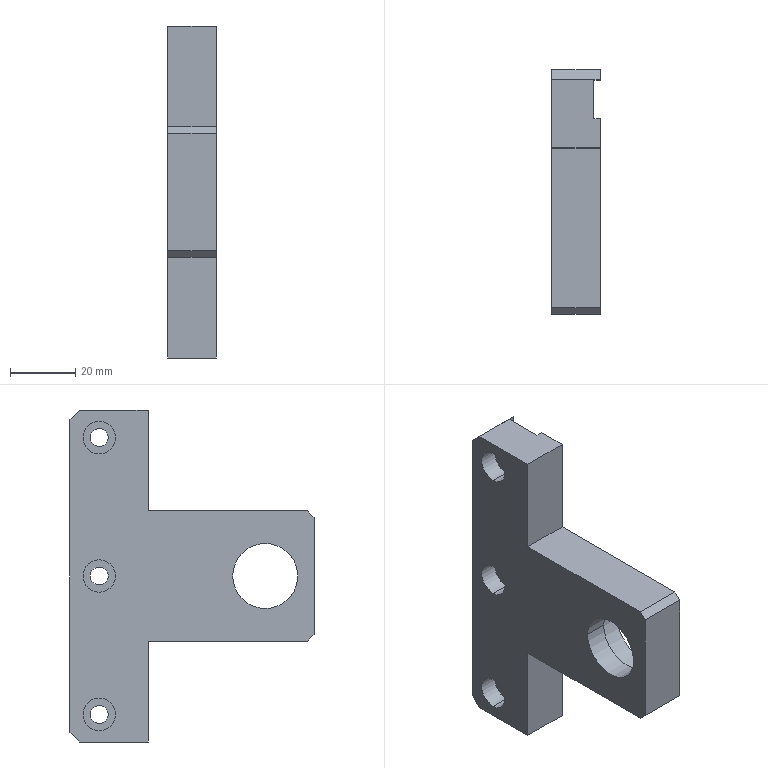Part | SolidWorks | features BaseBody 1 | 1 solid | 38 faces | box 15 x 75 x 102 mm | volume 56367 mm3 | plane 22 | cylinder 16 | commonest cylinder face diameters 5.5 x6 10 x6 20 x2 26 x2
STEP:
#1=CARTESIAN_POINT('',(-3.,-35.,-51.));
#2=VERTEX_POINT('',#1);
#3=CARTESIAN_POINT('',(-3.,-15.,-51.));
#4=VERTEX_POINT('',#3);
#5=CARTESIAN_POINT('',(-3.,-25.,-51.));
#6=DIRECTION('',(1.,0.,0.));
#7=DIRECTION('',(0.,1.,0.));
#8=AXIS2_PLACEMENT_3D('',#5,#6,#7);
#9=CIRCLE('',#8,10.);
#10=EDGE_CURVE('',#2,#4,#9,.T.);
#11=ORIENTED_EDGE('',*,*,#10,.F.);
#12=CARTESIAN_POINT('',(4.,-35.,-51.));
#13=VERTEX_POINT('',#12);
#14=CARTESIAN_POINT('',(-3.,-35.,-51.));
#15=DIRECTION('',(1.,0.,0.));
#16=VECTOR('',#15,1000.);
#17=LINE('',#14,#16);
#18=EDGE_CURVE('',#2,#13,#17,.T.);
#19=ORIENTED_EDGE('',*,*,#18,.T.);
#20=CARTESIAN_POINT('',(4.,-15.,-51.));
#21=VERTEX_POINT('',#20);
#22=CARTESIAN_POINT('',(4.,-25.,-51.));
#23=DIRECTION('',(-1.,0.,0.));
#24=DIRECTION('',(0.,1.,0.));
#25=AXIS2_PLACEMENT_3D('',#22,#23,#24);
#26=CIRCLE('',#25,10.);
#27=EDGE_CURVE('',#21,#13,#26,.T.);
#28=ORIENTED_EDGE('',*,*,#27,.F.);
#29=CARTESIAN_POINT('',(-3.,-15.,-51.));
#30=DIRECTION('',(1.,0.,0.));
#31=VECTOR('',#30,1000.);
#32=LINE('',#29,#31);
#33=EDGE_CURVE('',#4,#21,#32,.T.);
#34=ORIENTED_EDGE('',*,*,#33,.F.);
#35=EDGE_LOOP('',(#11,#19,#28,#34));
#36=FACE_OUTER_BOUND('',#35,.T.);
#37=CARTESIAN_POINT('',(-3.,-25.,-51.));
#38=DIRECTION('',(1.,0.,0.));
#39=DIRECTION('',(0.,1.,0.));
#40=AXIS2_PLACEMENT_3D('',#37,#38,#39);
#41=CYLINDRICAL_SURFACE('',#40,10.);
#42=ADVANCED_FACE('',(#36),#41,.F.);
#43=CARTESIAN_POINT('',(2.7,26.,-13.5));
#44=VERTEX_POINT('',#43);
#45=CARTESIAN_POINT('',(2.7,26.,-3.5));
#46=VERTEX_POINT('',#45);
#47=CARTESIAN_POINT('',(2.7,26.,-8.5));
#48=DIRECTION('',(-1.,0.,0.));
#49=DIRECTION('',(0.,0.,1.));
#50=AXIS2_PLACEMENT_3D('',#47,#48,#49);
#51=CIRCLE('',#50,5.);
#52=EDGE_CURVE('',#44,#46,#51,.T.);
#53=ORIENTED_EDGE('',*,*,#52,.F.);
#54=CARTESIAN_POINT('',(-3.,26.,-13.5));
#55=VERTEX_POINT('',#54);
#56=CARTESIAN_POINT('',(-3.,26.,-13.5));
#57=DIRECTION('',(-1.,0.,0.));
#58=VECTOR('',#57,1000.);
#59=LINE('',#56,#58);
#60=EDGE_CURVE('',#44,#55,#59,.T.);
#61=ORIENTED_EDGE('',*,*,#60,.T.);
#62=CARTESIAN_POINT('',(-3.,26.,-3.5));
#63=VERTEX_POINT('',#62);
#64=CARTESIAN_POINT('',(-3.,26.,-8.5));
#65=DIRECTION('',(1.,0.,0.));
#66=DIRECTION('',(0.,0.,1.));
#67=AXIS2_PLACEMENT_3D('',#64,#65,#66);
#68=CIRCLE('',#67,5.);
#69=EDGE_CURVE('',#63,#55,#68,.T.);
#70=ORIENTED_EDGE('',*,*,#69,.F.);
#71=CARTESIAN_POINT('',(-3.,26.,-3.5));
#72=DIRECTION('',(-1.,0.,0.));
#73=VECTOR('',#72,1000.);
#74=LINE('',#71,#73);
#75=EDGE_CURVE('',#46,#63,#74,.T.);
#76=ORIENTED_EDGE('',*,*,#75,.F.);
#77=EDGE_LOOP('',(#53,#61,#70,#76));
#78=FACE_OUTER_BOUND('',#77,.T.);
#79=CARTESIAN_POINT('',(-3.,26.,-8.5));
#80=DIRECTION('',(-1.,0.,0.));
#81=DIRECTION('',(0.,0.,1.));
#82=AXIS2_PLACEMENT_3D('',#79,#80,#81);
#83=CYLINDRICAL_SURFACE('',#82,5.);
#84=ADVANCED_FACE('',(#78),#83,.F.);
#85=CARTESIAN_POINT('',(2.7,26.,-56.));
#86=VERTEX_POINT('',#85);
#87=CARTESIAN_POINT('',(2.7,26.,-46.));
#88=VERTEX_POINT('',#87);
#89=CARTESIAN_POINT('',(2.7,26.,-51.));
#90=DIRECTION('',(-1.,0.,0.));
#91=DIRECTION('',(0.,0.,1.));
#92=AXIS2_PLACEMENT_3D('',#89,#90,#91);
#93=CIRCLE('',#92,5.);
#94=EDGE_CURVE('',#86,#88,#93,.T.);
#95=ORIENTED_EDGE('',*,*,#94,.F.);
#96=CARTESIAN_POINT('',(-3.,26.,-56.));
#97=VERTEX_POINT('',#96);
#98=CARTESIAN_POINT('',(-3.,26.,-56.));
#99=DIRECTION('',(-1.,0.,0.));
#100=VECTOR('',#99,1000.);
#101=LINE('',#98,#100);
#102=EDGE_CURVE('',#86,#97,#101,.T.);
#103=ORIENTED_EDGE('',*,*,#102,.T.);
#104=CARTESIAN_POINT('',(-3.,26.,-46.));
#105=VERTEX_POINT('',#104);
#106=CARTESIAN_POINT('',(-3.,26.,-51.));
#107=DIRECTION('',(1.,0.,0.));
#108=DIRECTION('',(0.,0.,1.));
#109=AXIS2_PLACEMENT_3D('',#106,#107,#108);
#110=CIRCLE('',#109,5.);
#111=EDGE_CURVE('',#105,#97,#110,.T.);
#112=ORIENTED_EDGE('',*,*,#111,.F.);
#113=CARTESIAN_POINT('',(-3.,26.,-46.));
#114=DIRECTION('',(-1.,0.,0.));
#115=VECTOR('',#114,1000.);
#116=LINE('',#113,#115);
#117=EDGE_CURVE('',#88,#105,#116,.T.);
#118=ORIENTED_EDGE('',*,*,#117,.F.);
#119=EDGE_LOOP('',(#95,#103,#112,#118));
#120=FACE_OUTER_BOUND('',#119,.T.);
#121=CARTESIAN_POINT('',(-3.,26.,-51.));
#122=DIRECTION('',(-1.,0.,0.));
#123=DIRECTION('',(0.,0.,1.));
#124=AXIS2_PLACEMENT_3D('',#121,#122,#123);
#125=CYLINDRICAL_SURFACE('',#124,5.);
#126=ADVANCED_FACE('',(#120),#125,.F.);
#127=CARTESIAN_POINT('',(2.7,26.,-98.5));
#128=VERTEX_POINT('',#127);
#129=CARTESIAN_POINT('',(2.7,26.,-88.5));
#130=VERTEX_POINT('',#129);
#131=CARTESIAN_POINT('',(2.7,26.,-93.5));
#132=DIRECTION('',(-1.,0.,0.));
#133=DIRECTION('',(0.,0.,1.));
#134=AXIS2_PLACEMENT_3D('',#131,#132,#133);
#135=CIRCLE('',#134,5.);
#136=EDGE_CURVE('',#128,#130,#135,.T.);
#137=ORIENTED_EDGE('',*,*,#136,.F.);
#138=CARTESIAN_POINT('',(-3.,26.,-98.5));
#139=VERTEX_POINT('',#138);
#140=CARTESIAN_POINT('',(-3.,26.,-98.5));
#141=DIRECTION('',(-1.,0.,0.));
#142=VECTOR('',#141,1000.);
#143=LINE('',#140,#142);
#144=EDGE_CURVE('',#128,#139,#143,.T.);
#145=ORIENTED_EDGE('',*,*,#144,.T.);
#146=CARTESIAN_POINT('',(-3.,26.,-88.5));
#147=VERTEX_POINT('',#146);
#148=CARTESIAN_POINT('',(-3.,26.,-93.5));
#149=DIRECTION('',(1.,0.,0.));
#150=DIRECTION('',(0.,0.,1.));
#151=AXIS2_PLACEMENT_3D('',#148,#149,#150);
#152=CIRCLE('',#151,5.);
#153=EDGE_CURVE('',#147,#139,#152,.T.);
#154=ORIENTED_EDGE('',*,*,#153,.F.);
#155=CARTESIAN_POINT('',(-3.,26.,-88.5));
#156=DIRECTION('',(-1.,0.,0.));
#157=VECTOR('',#156,1000.);
#158=LINE('',#155,#157);
#159=EDGE_CURVE('',#130,#147,#158,.T.);
#160=ORIENTED_EDGE('',*,*,#159,.F.);
#161=EDGE_LOOP('',(#137,#145,#154,#160));
#162=FACE_OUTER_BOUND('',#161,.T.);
#163=CARTESIAN_POINT('',(-3.,26.,-93.5));
#164=DIRECTION('',(-1.,0.,0.));
#165=DIRECTION('',(0.,0.,1.));
#166=AXIS2_PLACEMENT_3D('',#163,#164,#165);
#167=CYLINDRICAL_SURFACE('',#166,5.);
#168=ADVANCED_FACE('',(#162),#167,.F.);
#169=CARTESIAN_POINT('',(4.,-38.,-51.));
#170=VERTEX_POINT('',#169);
#171=CARTESIAN_POINT('',(4.,-12.,-51.));
#172=VERTEX_POINT('',#171);
#173=CARTESIAN_POINT('',(4.,-25.,-51.));
#174=DIRECTION('',(1.,0.,0.));
#175=DIRECTION('',(0.,1.,0.));
#176=AXIS2_PLACEMENT_3D('',#173,#174,#175);
#177=CIRCLE('',#176,13.);
#178=EDGE_CURVE('',#170,#172,#177,.T.);
#179=ORIENTED_EDGE('',*,*,#178,.F.);
#180=CARTESIAN_POINT('',(12.,-38.,-51.));
#181=VERTEX_POINT('',#180);
#182=CARTESIAN_POINT('',(4.,-38.,-51.));
#183=DIRECTION('',(1.,0.,0.));
#184=VECTOR('',#183,1000.);
#185=LINE('',#182,#184);
#186=EDGE_CURVE('',#170,#181,#185,.T.);
#187=ORIENTED_EDGE('',*,*,#186,.T.);
#188=CARTESIAN_POINT('',(12.,-12.,-51.));
#189=VERTEX_POINT('',#188);
#190=CARTESIAN_POINT('',(12.,-25.,-51.));
#191=DIRECTION('',(-1.,0.,0.));
#192=DIRECTION('',(0.,1.,0.));
#193=AXIS2_PLACEMENT_3D('',#190,#191,#192);
#194=CIRCLE('',#193,13.);
#195=EDGE_CURVE('',#189,#181,#194,.T.);
#196=ORIENTED_EDGE('',*,*,#195,.F.);
#197=CARTESIAN_POINT('',(4.,-12.,-51.));
#198=DIRECTION('',(1.,0.,0.));
#199=VECTOR('',#198,1000.);
#200=LINE('',#197,#199);
#201=EDGE_CURVE('',#172,#189,#200,.T.);
#202=ORIENTED_EDGE('',*,*,#201,.F.);
#203=EDGE_LOOP('',(#179,#187,#196,#202));
#204=FACE_OUTER_BOUND('',#203,.T.);
#205=CARTESIAN_POINT('',(4.,-25.,-51.));
#206=DIRECTION('',(1.,0.,0.));
#207=DIRECTION('',(0.,1.,0.));
#208=AXIS2_PLACEMENT_3D('',#205,#206,#207);
#209=CYLINDRICAL_SURFACE('',#208,13.);
#210=ADVANCED_FACE('',(#204),#209,.F.);
#211=CARTESIAN_POINT('',(10.,26.,-5.75));
#212=VERTEX_POINT('',#211);
#213=CARTESIAN_POINT('',(10.,26.,-11.25));
#214=VERTEX_POINT('',#213);
#215=CARTESIAN_POINT('',(10.,26.,-8.5));
#216=DIRECTION('',(1.,0.,0.));
#217=DIRECTION('',(0.,0.,1.));
#218=AXIS2_PLACEMENT_3D('',#215,#216,#217);
#219=CIRCLE('',#218,2.75);
#220=EDGE_CURVE('',#212,#214,#219,.T.);
#221=ORIENTED_EDGE('',*,*,#220,.T.);
#222=CARTESIAN_POINT('',(2.7,26.,-11.25));
#223=VERTEX_POINT('',#222);
#224=CARTESIAN_POINT('',(-3.,26.,-11.25));
#225=DIRECTION('',(-1.,0.,0.));
#226=VECTOR('',#225,1000.);
#227=LINE('',#224,#226);
#228=EDGE_CURVE('',#214,#223,#227,.T.);
#229=ORIENTED_EDGE('',*,*,#228,.T.);
#230=CARTESIAN_POINT('',(2.7,26.,-5.75));
#231=VERTEX_POINT('',#230);
#232=CARTESIAN_POINT('',(2.7,26.,-8.5));
#233=DIRECTION('',(-1.,0.,0.));
#234=DIRECTION('',(0.,0.,1.));
#235=AXIS2_PLACEMENT_3D('',#232,#233,#234);
#236=CIRCLE('',#235,2.75);
#237=EDGE_CURVE('',#223,#231,#236,.T.);
#238=ORIENTED_EDGE('',*,*,#237,.T.);
#239=CARTESIAN_POINT('',(-3.,26.,-5.75));
#240=DIRECTION('',(-1.,0.,0.));
#241=VECTOR('',#240,1000.);
#242=LINE('',#239,#241);
#243=EDGE_CURVE('',#212,#231,#242,.T.);
#244=ORIENTED_EDGE('',*,*,#243,.F.);
#245=EDGE_LOOP('',(#221,#229,#238,#244));
#246=FACE_OUTER_BOUND('',#245,.T.);
#247=CARTESIAN_POINT('',(-3.,26.,-8.5));
#248=DIRECTION('',(-1.,0.,0.));
#249=DIRECTION('',(0.,0.,1.));
#250=AXIS2_PLACEMENT_3D('',#247,#248,#249);
#251=CYLINDRICAL_SURFACE('',#250,2.75);
#252=ADVANCED_FACE('',(#246),#251,.F.);
#253=CARTESIAN_POINT('',(10.,26.,-48.25));
#254=VERTEX_POINT('',#253);
#255=CARTESIAN_POINT('',(10.,26.,-53.75));
#256=VERTEX_POINT('',#255);
#257=CARTESIAN_POINT('',(10.,26.,-51.));
#258=DIRECTION('',(1.,0.,0.));
#259=DIRECTION('',(0.,0.,1.));
#260=AXIS2_PLACEMENT_3D('',#257,#258,#259);
#261=CIRCLE('',#260,2.75);
#262=EDGE_CURVE('',#254,#256,#261,.T.);
#263=ORIENTED_EDGE('',*,*,#262,.T.);
#264=CARTESIAN_POINT('',(2.7,26.,-53.75));
#265=VERTEX_POINT('',#264);
#266=CARTESIAN_POINT('',(-3.,26.,-53.75));
#267=DIRECTION('',(-1.,0.,0.));
#268=VECTOR('',#267,1000.);
#269=LINE('',#266,#268);
#270=EDGE_CURVE('',#256,#265,#269,.T.);
#271=ORIENTED_EDGE('',*,*,#270,.T.);
#272=CARTESIAN_POINT('',(2.7,26.,-48.25));
#273=VERTEX_POINT('',#272);
#274=CARTESIAN_POINT('',(2.7,26.,-51.));
#275=DIRECTION('',(-1.,0.,0.));
#276=DIRECTION('',(0.,0.,1.));
#277=AXIS2_PLACEMENT_3D('',#274,#275,#276);
#278=CIRCLE('',#277,2.75);
#279=EDGE_CURVE('',#265,#273,#278,.T.);
#280=ORIENTED_EDGE('',*,*,#279,.T.);
#281=CARTESIAN_POINT('',(-3.,26.,-48.25));
#282=DIRECTION('',(-1.,0.,0.));
#283=VECTOR('',#282,1000.);
#284=LINE('',#281,#283);
#285=EDGE_CURVE('',#254,#273,#284,.T.);
#286=ORIENTED_EDGE('',*,*,#285,.F.);
#287=EDGE_LOOP('',(#263,#271,#280,#286));
#288=FACE_OUTER_BOUND('',#287,.T.);
#289=CARTESIAN_POINT('',(-3.,26.,-51.));
#290=DIRECTION('',(-1.,0.,0.));
#291=DIRECTION('',(0.,0.,1.));
#292=AXIS2_PLACEMENT_3D('',#289,#290,#291);
#293=CYLINDRICAL_SURFACE('',#292,2.75);
#294=ADVANCED_FACE('',(#288),#293,.F.);
#295=CARTESIAN_POINT('',(10.,26.,-90.75));
#296=VERTEX_POINT('',#295);
#297=CARTESIAN_POINT('',(10.,26.,-96.25));
#298=VERTEX_POINT('',#297);
#299=CARTESIAN_POINT('',(10.,26.,-93.5));
#300=DIRECTION('',(1.,0.,0.));
#301=DIRECTION('',(0.,0.,1.));
#302=AXIS2_PLACEMENT_3D('',#299,#300,#301);
#303=CIRCLE('',#302,2.75);
#304=EDGE_CURVE('',#296,#298,#303,.T.);
#305=ORIENTED_EDGE('',*,*,#304,.T.);
#306=CARTESIAN_POINT('',(2.7,26.,-96.25));
#307=VERTEX_POINT('',#306);
#308=CARTESIAN_POINT('',(-3.,26.,-96.25));
#309=DIRECTION('',(-1.,0.,0.));
#310=VECTOR('',#309,1000.);
#311=LINE('',#308,#310);
#312=EDGE_CURVE('',#298,#307,#311,.T.);
#313=ORIENTED_EDGE('',*,*,#312,.T.);
#314=CARTESIAN_POINT('',(2.7,26.,-90.75));
#315=VERTEX_POINT('',#314);
#316=CARTESIAN_POINT('',(2.7,26.,-93.5));
#317=DIRECTION('',(-1.,0.,0.));
#318=DIRECTION('',(0.,0.,1.));
#319=AXIS2_PLACEMENT_3D('',#316,#317,#318);
#320=CIRCLE('',#319,2.75);
#321=EDGE_CURVE('',#307,#315,#320,.T.);
#322=ORIENTED_EDGE('',*,*,#321,.T.);
#323=CARTESIAN_POINT('',(-3.,26.,-90.75));
#324=DIRECTION('',(-1.,0.,0.));
#325=VECTOR('',#324,1000.);
#326=LINE('',#323,#325);
#327=EDGE_CURVE('',#296,#315,#326,.T.);
#328=ORIENTED_EDGE('',*,*,#327,.F.);
#329=EDGE_LOOP('',(#305,#313,#322,#328));
#330=FACE_OUTER_BOUND('',#329,.T.);
#331=CARTESIAN_POINT('',(-3.,26.,-93.5));
#332=DIRECTION('',(-1.,0.,0.));
#333=DIRECTION('',(0.,0.,1.));
#334=AXIS2_PLACEMENT_3D('',#331,#332,#333);
#335=CYLINDRICAL_SURFACE('',#334,2.75);
#336=ADVANCED_FACE('',(#330),#335,.F.);
#337=CARTESIAN_POINT('',(-3.,-25.,-51.));
#338=DIRECTION('',(1.,0.,0.));
#339=DIRECTION('',(0.,1.,0.));
#340=AXIS2_PLACEMENT_3D('',#337,#338,#339);
#341=CIRCLE('',#340,10.);
#342=EDGE_CURVE('',#4,#2,#341,.T.);
#343=ORIENTED_EDGE('',*,*,#342,.T.);
#344=ORIENTED_EDGE('',*,*,#10,.T.);
#345=EDGE_LOOP('',(#343,#344));
#346=FACE_BOUND('',#345,.T.);
#347=ORIENTED_EDGE('',*,*,#69,.T.);
#348=CARTESIAN_POINT('',(-3.,26.,-8.5));
#349=DIRECTION('',(1.,0.,0.));
#350=DIRECTION('',(0.,0.,1.));
#351=AXIS2_PLACEMENT_3D('',#348,#349,#350);
#352=CIRCLE('',#351,5.);
#353=EDGE_CURVE('',#55,#63,#352,.T.);
#354=ORIENTED_EDGE('',*,*,#353,.T.);
#355=EDGE_LOOP('',(#347,#354));
#356=FACE_BOUND('',#355,.T.);
#357=ORIENTED_EDGE('',*,*,#111,.T.);
#358=CARTESIAN_POINT('',(-3.,26.,-51.));
#359=DIRECTION('',(1.,0.,0.));
#360=DIRECTION('',(0.,0.,1.));
#361=AXIS2_PLACEMENT_3D('',#358,#359,#360);
#362=CIRCLE('',#361,5.);
#363=EDGE_CURVE('',#97,#105,#362,.T.);
#364=ORIENTED_EDGE('',*,*,#363,.T.);
#365=EDGE_LOOP('',(#357,#364));
#366=FACE_BOUND('',#365,.T.);
#367=ORIENTED_EDGE('',*,*,#153,.T.);
#368=CARTESIAN_POINT('',(-3.,26.,-93.5));
#369=DIRECTION('',(1.,0.,0.));
#370=DIRECTION('',(0.,0.,1.));
#371=AXIS2_PLACEMENT_3D('',#368,#369,#370);
#372=CIRCLE('',#371,5.);
#373=EDGE_CURVE('',#139,#147,#372,.T.);
#374=ORIENTED_EDGE('',*,*,#373,.T.);
#375=EDGE_LOOP('',(#367,#374));
#376=FACE_BOUND('',#375,.T.);
#377=CARTESIAN_POINT('',(-3.,11.,-71.));
#378=VERTEX_POINT('',#377);
#379=CARTESIAN_POINT('',(-3.,-38.,-71.));
#380=VERTEX_POINT('',#379);
#381=CARTESIAN_POINT('',(-3.,35.,-71.));
#382=DIRECTION('',(0.,-1.,0.));
#383=VECTOR('',#382,1000.);
#384=LINE('',#381,#383);
#385=EDGE_CURVE('',#378,#380,#384,.T.);
#386=ORIENTED_EDGE('',*,*,#385,.T.);
#387=CARTESIAN_POINT('',(-3.,-40.,-69.));
#388=VERTEX_POINT('',#387);
#389=CARTESIAN_POINT('',(-3.,-38.,-71.));
#390=DIRECTION('',(0.,-0.7071,0.7071));
#391=VECTOR('',#390,1000.);
#392=LINE('',#389,#391);
#393=EDGE_CURVE('',#380,#388,#392,.T.);
#394=ORIENTED_EDGE('',*,*,#393,.T.);
#395=CARTESIAN_POINT('',(-3.,-40.,-33.));
#396=VERTEX_POINT('',#395);
#397=CARTESIAN_POINT('',(-3.,-40.,-102.));
#398=DIRECTION('',(0.,0.,1.));
#399=VECTOR('',#398,1000.);
#400=LINE('',#397,#399);
#401=EDGE_CURVE('',#388,#396,#400,.T.);
#402=ORIENTED_EDGE('',*,*,#401,.T.);
#403=CARTESIAN_POINT('',(-3.,-38.,-31.));
#404=VERTEX_POINT('',#403);
#405=CARTESIAN_POINT('',(-3.,-40.,-33.));
#406=DIRECTION('',(0.,0.7071,0.7071));
#407=VECTOR('',#406,1000.);
#408=LINE('',#405,#407);
#409=EDGE_CURVE('',#396,#404,#408,.T.);
#410=ORIENTED_EDGE('',*,*,#409,.T.);
#411=CARTESIAN_POINT('',(-3.,11.,-31.));
#412=VERTEX_POINT('',#411);
#413=CARTESIAN_POINT('',(-3.,35.,-31.));
#414=DIRECTION('',(0.,1.,0.));
#415=VECTOR('',#414,1000.);
#416=LINE('',#413,#415);
#417=EDGE_CURVE('',#404,#412,#416,.T.);
#418=ORIENTED_EDGE('',*,*,#417,.T.);
#419=CARTESIAN_POINT('',(-3.,11.,0.));
#420=VERTEX_POINT('',#419);
#421=CARTESIAN_POINT('',(-3.,11.,-102.));
#422=DIRECTION('',(0.,0.,1.));
#423=VECTOR('',#422,1000.);
#424=LINE('',#421,#423);
#425=EDGE_CURVE('',#412,#420,#424,.T.);
#426=ORIENTED_EDGE('',*,*,#425,.T.);
#427=CARTESIAN_POINT('',(-3.,32.,0.));
#428=VERTEX_POINT('',#427);
#429=CARTESIAN_POINT('',(-3.,35.,0.));
#430=DIRECTION('',(0.,1.,0.));
#431=VECTOR('',#430,1000.);
#432=LINE('',#429,#431);
#433=EDGE_CURVE('',#420,#428,#432,.T.);
#434=ORIENTED_EDGE('',*,*,#433,.T.);
#435=CARTESIAN_POINT('',(-3.,35.,-3.));
#436=VERTEX_POINT('',#435);
#437=CARTESIAN_POINT('',(-3.,32.,0.));
#438=DIRECTION('',(0.,0.7071,-0.7071));
#439=VECTOR('',#438,1000.);
#440=LINE('',#437,#439);
#441=EDGE_CURVE('',#428,#436,#440,.T.);
#442=ORIENTED_EDGE('',*,*,#441,.T.);
#443=CARTESIAN_POINT('',(-3.,35.,-99.));
#444=VERTEX_POINT('',#443);
#445=CARTESIAN_POINT('',(-3.,35.,-102.));
#446=DIRECTION('',(0.,0.,-1.));
#447=VECTOR('',#446,1000.);
#448=LINE('',#445,#447);
#449=EDGE_CURVE('',#436,#444,#448,.T.);
#450=ORIENTED_EDGE('',*,*,#449,.T.);
#451=CARTESIAN_POINT('',(-3.,32.,-102.));
#452=VERTEX_POINT('',#451);
#453=CARTESIAN_POINT('',(-3.,35.,-99.));
#454=DIRECTION('',(0.,-0.7071,-0.7071));
#455=VECTOR('',#454,1000.);
#456=LINE('',#453,#455);
#457=EDGE_CURVE('',#444,#452,#456,.T.);
#458=ORIENTED_EDGE('',*,*,#457,.T.);
#459=CARTESIAN_POINT('',(-3.,11.,-102.));
#460=VERTEX_POINT('',#459);
#461=CARTESIAN_POINT('',(-3.,35.,-102.));
#462=DIRECTION('',(0.,-1.,0.));
#463=VECTOR('',#462,1000.);
#464=LINE('',#461,#463);
#465=EDGE_CURVE('',#452,#460,#464,.T.);
#466=ORIENTED_EDGE('',*,*,#465,.T.);
#467=CARTESIAN_POINT('',(-3.,11.,-102.));
#468=DIRECTION('',(0.,0.,1.));
#469=VECTOR('',#468,1000.);
#470=LINE('',#467,#469);
#471=EDGE_CURVE('',#460,#378,#470,.T.);
#472=ORIENTED_EDGE('',*,*,#471,.T.);
#473=EDGE_LOOP('',(#386,#394,#402,#410,#418,#426,#434,#442,#450,#458,#466,#472));
#474=FACE_OUTER_BOUND('',#473,.T.);
#475=CARTESIAN_POINT('',(-3.,35.,-102.));
#476=DIRECTION('',(-1.,0.,0.));
#477=DIRECTION('',(0.,-1.,0.));
#478=AXIS2_PLACEMENT_3D('',#475,#476,#477);
#479=PLANE('',#478);
#480=ADVANCED_FACE('',(#346,#356,#366,#376,#474),#479,.T.);
#481=ORIENTED_EDGE('',*,*,#18,.F.);
#482=ORIENTED_EDGE('',*,*,#342,.F.);
#483=ORIENTED_EDGE('',*,*,#33,.T.);
#484=CARTESIAN_POINT('',(4.,-25.,-51.));
#485=DIRECTION('',(-1.,0.,0.));
#486=DIRECTION('',(0.,1.,0.));
#487=AXIS2_PLACEMENT_3D('',#484,#485,#486);
#488=CIRCLE('',#487,10.);
#489=EDGE_CURVE('',#13,#21,#488,.T.);
#490=ORIENTED_EDGE('',*,*,#489,.F.);
#491=EDGE_LOOP('',(#481,#482,#483,#490));
#492=FACE_OUTER_BOUND('',#491,.T.);
#493=CARTESIAN_POINT('',(-3.,-25.,-51.));
#494=DIRECTION('',(1.,0.,0.));
#495=DIRECTION('',(0.,1.,0.));
#496=AXIS2_PLACEMENT_3D('',#493,#494,#495);
#497=CYLINDRICAL_SURFACE('',#496,10.);
#498=ADVANCED_FACE('',(#492),#497,.F.);
#499=ORIENTED_EDGE('',*,*,#60,.F.);
#500=CARTESIAN_POINT('',(2.7,26.,-8.5));
#501=DIRECTION('',(-1.,0.,0.));
#502=DIRECTION('',(0.,0.,1.));
#503=AXIS2_PLACEMENT_3D('',#500,#501,#502);
#504=CIRCLE('',#503,5.);
#505=EDGE_CURVE('',#46,#44,#504,.T.);
#506=ORIENTED_EDGE('',*,*,#505,.F.);
#507=ORIENTED_EDGE('',*,*,#75,.T.);
#508=ORIENTED_EDGE('',*,*,#353,.F.);
#509=EDGE_LOOP('',(#499,#506,#507,#508));
#510=FACE_OUTER_BOUND('',#509,.T.);
#511=CARTESIAN_POINT('',(-3.,26.,-8.5));
#512=DIRECTION('',(-1.,0.,0.));
#513=DIRECTION('',(0.,0.,1.));
#514=AXIS2_PLACEMENT_3D('',#511,#512,#513);
#515=CYLINDRICAL_SURFACE('',#514,5.);
#516=ADVANCED_FACE('',(#510),#515,.F.);
#517=ORIENTED_EDGE('',*,*,#102,.F.);
#518=CARTESIAN_POINT('',(2.7,26.,-51.));
#519=DIRECTION('',(-1.,0.,0.));
#520=DIRECTION('',(0.,0.,1.));
#521=AXIS2_PLACEMENT_3D('',#518,#519,#520);
#522=CIRCLE('',#521,5.);
#523=EDGE_CURVE('',#88,#86,#522,.T.);
#524=ORIENTED_EDGE('',*,*,#523,.F.);
#525=ORIENTED_EDGE('',*,*,#117,.T.);
#526=ORIENTED_EDGE('',*,*,#363,.F.);
#527=EDGE_LOOP('',(#517,#524,#525,#526));
#528=FACE_OUTER_BOUND('',#527,.T.);
#529=CARTESIAN_POINT('',(-3.,26.,-51.));
#530=DIRECTION('',(-1.,0.,0.));
#531=DIRECTION('',(0.,0.,1.));
#532=AXIS2_PLACEMENT_3D('',#529,#530,#531);
#533=CYLINDRICAL_SURFACE('',#532,5.);
#534=ADVANCED_FACE('',(#528),#533,.F.);
#535=ORIENTED_EDGE('',*,*,#144,.F.);
#536=CARTESIAN_POINT('',(2.7,26.,-93.5));
#537=DIRECTION('',(-1.,0.,0.));
#538=DIRECTION('',(0.,0.,1.));
#539=AXIS2_PLACEMENT_3D('',#536,#537,#538);
#540=CIRCLE('',#539,5.);
#541=EDGE_CURVE('',#130,#128,#540,.T.);
#542=ORIENTED_EDGE('',*,*,#541,.F.);
#543=ORIENTED_EDGE('',*,*,#159,.T.);
#544=ORIENTED_EDGE('',*,*,#373,.F.);
#545=EDGE_LOOP('',(#535,#542,#543,#544));
#546=FACE_OUTER_BOUND('',#545,.T.);
#547=CARTESIAN_POINT('',(-3.,26.,-93.5));
#548=DIRECTION('',(-1.,0.,0.));
#549=DIRECTION('',(0.,0.,1.));
#550=AXIS2_PLACEMENT_3D('',#547,#548,#549);
#551=CYLINDRICAL_SURFACE('',#550,5.);
#552=ADVANCED_FACE('',(#546),#551,.F.);
#553=ORIENTED_EDGE('',*,*,#393,.F.);
#554=CARTESIAN_POINT('',(12.,-38.,-71.));
#555=VERTEX_POINT('',#554);
#556=CARTESIAN_POINT('',(-3.,-38.,-71.));
#557=DIRECTION('',(1.,0.,0.));
#558=VECTOR('',#557,1000.);
#559=LINE('',#556,#558);
#560=EDGE_CURVE('',#380,#555,#559,.T.);
#561=ORIENTED_EDGE('',*,*,#560,.T.);
#562=CARTESIAN_POINT('',(12.,-40.,-69.));
#563=VERTEX_POINT('',#562);
#564=CARTESIAN_POINT('',(12.,-38.,-71.));
#565=DIRECTION('',(0.,-0.7071,0.7071));
#566=VECTOR('',#565,1000.);
#567=LINE('',#564,#566);
#568=EDGE_CURVE('',#555,#563,#567,.T.);
#569=ORIENTED_EDGE('',*,*,#568,.T.);
#570=CARTESIAN_POINT('',(-3.,-40.,-69.));
#571=DIRECTION('',(-1.,0.,0.));
#572=VECTOR('',#571,1000.);
#573=LINE('',#570,#572);
#574=EDGE_CURVE('',#563,#388,#573,.T.);
#575=ORIENTED_EDGE('',*,*,#574,.T.);
#576=EDGE_LOOP('',(#553,#561,#569,#575));
#577=FACE_OUTER_BOUND('',#576,.T.);
#578=CARTESIAN_POINT('',(-3.,-38.,-71.));
#579=DIRECTION('',(0.,-0.7071,-0.7071));
#580=DIRECTION('',(0.,0.7071,-0.7071));
#581=AXIS2_PLACEMENT_3D('',#578,#579,#580);
#582=PLANE('',#581);
#583=ADVANCED_FACE('',(#577),#582,.T.);
#584=ORIENTED_EDGE('',*,*,#560,.F.);
#585=ORIENTED_EDGE('',*,*,#385,.F.);
#586=CARTESIAN_POINT('',(12.,11.,-71.));
#587=VERTEX_POINT('',#586);
#588=CARTESIAN_POINT('',(-3.,11.,-71.));
#589=DIRECTION('',(-1.,0.,0.));
#590=VECTOR('',#589,1000.);
#591=LINE('',#588,#590);
#592=EDGE_CURVE('',#587,#378,#591,.T.);
#593=ORIENTED_EDGE('',*,*,#592,.F.);
#594=CARTESIAN_POINT('',(12.,11.,-71.));
#595=DIRECTION('',(0.,1.,0.));
#596=VECTOR('',#595,1000.);
#597=LINE('',#594,#596);
#598=EDGE_CURVE('',#555,#587,#597,.T.);
#599=ORIENTED_EDGE('',*,*,#598,.F.);
#600=EDGE_LOOP('',(#584,#585,#593,#599));
#601=FACE_OUTER_BOUND('',#600,.T.);
#602=CARTESIAN_POINT('',(-3.,11.,-71.));
#603=DIRECTION('',(0.,0.,1.));
#604=DIRECTION('',(0.,-1.,0.));
#605=AXIS2_PLACEMENT_3D('',#602,#603,#604);
#606=PLANE('',#605);
#607=ADVANCED_FACE('',(#601),#606,.F.);
#608=ORIENTED_EDGE('',*,*,#592,.T.);
#609=ORIENTED_EDGE('',*,*,#471,.F.);
#610=CARTESIAN_POINT('',(12.,11.,-102.));
#611=VERTEX_POINT('',#610);
#612=CARTESIAN_POINT('',(-3.,11.,-102.));
#613=DIRECTION('',(-1.,0.,0.));
#614=VECTOR('',#613,1000.);
#615=LINE('',#612,#614);
#616=EDGE_CURVE('',#611,#460,#615,.T.);
#617=ORIENTED_EDGE('',*,*,#616,.F.);
#618=CARTESIAN_POINT('',(12.,11.,-102.));
#619=DIRECTION('',(0.,0.,-1.));
#620=VECTOR('',#619,1000.);
#621=LINE('',#618,#620);
#622=EDGE_CURVE('',#587,#611,#621,.T.);
#623=ORIENTED_EDGE('',*,*,#622,.F.);
#624=EDGE_LOOP('',(#608,#609,#617,#623));
#625=FACE_OUTER_BOUND('',#624,.T.);
#626=CARTESIAN_POINT('',(-3.,11.,-102.));
#627=DIRECTION('',(0.,1.,0.));
#628=DIRECTION('',(-1.,0.,0.));
#629=AXIS2_PLACEMENT_3D('',#626,#627,#628);
#630=PLANE('',#629);
#631=ADVANCED_FACE('',(#625),#630,.F.);
#632=ORIENTED_EDGE('',*,*,#616,.T.);
#633=ORIENTED_EDGE('',*,*,#465,.F.);
#634=CARTESIAN_POINT('',(10.,32.,-102.));
#635=VERTEX_POINT('',#634);
#636=CARTESIAN_POINT('',(0.,32.,-102.));
#637=DIRECTION('',(-1.,0.,0.));
#638=VECTOR('',#637,1000.);
#639=LINE('',#636,#638);
#640=EDGE_CURVE('',#635,#452,#639,.T.);
#641=ORIENTED_EDGE('',*,*,#640,.F.);
#642=CARTESIAN_POINT('',(10.,20.,-102.));
#643=VERTEX_POINT('',#642);
#644=CARTESIAN_POINT('',(10.,0.,-102.));
#645=DIRECTION('',(0.,1.,0.));
#646=VECTOR('',#645,1000.);
#647=LINE('',#644,#646);
#648=EDGE_CURVE('',#643,#635,#647,.T.);
#649=ORIENTED_EDGE('',*,*,#648,.F.);
#650=CARTESIAN_POINT('',(12.,20.,-102.));
#651=VERTEX_POINT('',#650);
#652=CARTESIAN_POINT('',(0.,20.,-102.));
#653=DIRECTION('',(-1.,0.,0.));
#654=VECTOR('',#653,1000.);
#655=LINE('',#652,#654);
#656=EDGE_CURVE('',#651,#643,#655,.T.);
#657=ORIENTED_EDGE('',*,*,#656,.F.);
#658=CARTESIAN_POINT('',(12.,0.,-102.));
#659=DIRECTION('',(0.,1.,0.));
#660=VECTOR('',#659,1000.);
#661=LINE('',#658,#660);
#662=EDGE_CURVE('',#611,#651,#661,.T.);
#663=ORIENTED_EDGE('',*,*,#662,.F.);
#664=EDGE_LOOP('',(#632,#633,#641,#649,#657,#663));
#665=FACE_OUTER_BOUND('',#664,.T.);
#666=CARTESIAN_POINT('',(0.,0.,-102.));
#667=DIRECTION('',(0.,0.,1.));
#668=DIRECTION('',(1.,0.,0.));
#669=AXIS2_PLACEMENT_3D('',#666,#667,#668);
#670=PLANE('',#669);
#671=ADVANCED_FACE('',(#665),#670,.F.);
#672=CARTESIAN_POINT('',(12.,35.,-99.));
#673=VERTEX_POINT('',#672);
#674=CARTESIAN_POINT('',(-3.,35.,-99.));
#675=DIRECTION('',(1.,0.,0.));
#676=VECTOR('',#675,1000.);
#677=LINE('',#674,#676);
#678=EDGE_CURVE('',#444,#673,#677,.T.);
#679=ORIENTED_EDGE('',*,*,#678,.T.);
#680=CARTESIAN_POINT('',(12.,32.,-102.));
#681=VERTEX_POINT('',#680);
#682=CARTESIAN_POINT('',(12.,35.,-99.));
#683=DIRECTION('',(0.,-0.7071,-0.7071));
#684=VECTOR('',#683,1000.);
#685=LINE('',#682,#684);
#686=EDGE_CURVE('',#673,#681,#685,.T.);
#687=ORIENTED_EDGE('',*,*,#686,.T.);
#688=CARTESIAN_POINT('',(-3.,32.,-102.));
#689=DIRECTION('',(-1.,0.,0.));
#690=VECTOR('',#689,1000.);
#691=LINE('',#688,#690);
#692=EDGE_CURVE('',#681,#635,#691,.T.);
#693=ORIENTED_EDGE('',*,*,#692,.T.);
#694=ORIENTED_EDGE('',*,*,#640,.T.);
#695=ORIENTED_EDGE('',*,*,#457,.F.);
#696=EDGE_LOOP('',(#679,#687,#693,#694,#695));
#697=FACE_OUTER_BOUND('',#696,.T.);
#698=CARTESIAN_POINT('',(-3.,35.,-99.));
#699=DIRECTION('',(0.,0.7071,-0.7071));
#700=DIRECTION('',(0.,0.7071,0.7071));
#701=AXIS2_PLACEMENT_3D('',#698,#699,#700);
#702=PLANE('',#701);
#703=ADVANCED_FACE('',(#697),#702,.T.);
#704=CARTESIAN_POINT('',(12.,35.,-3.));
#705=VERTEX_POINT('',#704);
#706=CARTESIAN_POINT('',(12.,35.,-102.));
#707=DIRECTION('',(0.,0.,-1.));
#708=VECTOR('',#707,1000.);
#709=LINE('',#706,#708);
#710=EDGE_CURVE('',#705,#673,#709,.T.);
#711=ORIENTED_EDGE('',*,*,#710,.T.);
#712=ORIENTED_EDGE('',*,*,#678,.F.);
#713=ORIENTED_EDGE('',*,*,#449,.F.);
#714=CARTESIAN_POINT('',(-3.,35.,-3.));
#715=DIRECTION('',(1.,0.,0.));
#716=VECTOR('',#715,1000.);
#717=LINE('',#714,#716);
#718=EDGE_CURVE('',#436,#705,#717,.T.);
#719=ORIENTED_EDGE('',*,*,#718,.T.);
#720=EDGE_LOOP('',(#711,#712,#713,#719));
#721=FACE_OUTER_BOUND('',#720,.T.);
#722=CARTESIAN_POINT('',(-3.,35.,-102.));
#723=DIRECTION('',(0.,1.,0.));
#724=DIRECTION('',(0.,0.,1.));
#725=AXIS2_PLACEMENT_3D('',#722,#723,#724);
#726=PLANE('',#725);
#727=ADVANCED_FACE('',(#721),#726,.T.);
#728=ORIENTED_EDGE('',*,*,#718,.F.);
#729=ORIENTED_EDGE('',*,*,#441,.F.);
#730=CARTESIAN_POINT('',(10.,32.,0.));
#731=VERTEX_POINT('',#730);
#732=CARTESIAN_POINT('',(0.,32.,0.));
#733=DIRECTION('',(-1.,0.,0.));
#734=VECTOR('',#733,1000.);
#735=LINE('',#732,#734);
#736=EDGE_CURVE('',#731,#428,#735,.T.);
#737=ORIENTED_EDGE('',*,*,#736,.F.);
#738=CARTESIAN_POINT('',(12.,32.,0.));
#739=VERTEX_POINT('',#738);
#740=CARTESIAN_POINT('',(0.,32.,0.));
#741=DIRECTION('',(-1.,0.,0.));
#742=VECTOR('',#741,1000.);
#743=LINE('',#740,#742);
#744=EDGE_CURVE('',#739,#731,#743,.T.);
#745=ORIENTED_EDGE('',*,*,#744,.F.);
#746=CARTESIAN_POINT('',(12.,32.,0.));
#747=DIRECTION('',(0.,-0.7071,0.7071));
#748=VECTOR('',#747,1000.);
#749=LINE('',#746,#748);
#750=EDGE_CURVE('',#705,#739,#749,.T.);
#751=ORIENTED_EDGE('',*,*,#750,.F.);
#752=EDGE_LOOP('',(#728,#729,#737,#745,#751));
#753=FACE_OUTER_BOUND('',#752,.T.);
#754=CARTESIAN_POINT('',(0.,32.,0.));
#755=DIRECTION('',(0.,-0.7071,-0.7071));
#756=DIRECTION('',(0.,0.7071,-0.7071));
#757=AXIS2_PLACEMENT_3D('',#754,#755,#756);
#758=PLANE('',#757);
#759=ADVANCED_FACE('',(#753),#758,.F.);
#760=ORIENTED_EDGE('',*,*,#736,.T.);
#761=ORIENTED_EDGE('',*,*,#433,.F.);
#762=CARTESIAN_POINT('',(12.,11.,0.));
#763=VERTEX_POINT('',#762);
#764=CARTESIAN_POINT('',(0.,11.,0.));
#765=DIRECTION('',(1.,0.,0.));
#766=VECTOR('',#765,1000.);
#767=LINE('',#764,#766);
#768=EDGE_CURVE('',#420,#763,#767,.T.);
#769=ORIENTED_EDGE('',*,*,#768,.T.);
#770=CARTESIAN_POINT('',(12.,20.,0.));
#771=VERTEX_POINT('',#770);
#772=CARTESIAN_POINT('',(12.,0.,0.));
#773=DIRECTION('',(0.,1.,0.));
#774=VECTOR('',#773,1000.);
#775=LINE('',#772,#774);
#776=EDGE_CURVE('',#763,#771,#775,.T.);
#777=ORIENTED_EDGE('',*,*,#776,.T.);
#778=CARTESIAN_POINT('',(10.,20.,0.));
#779=VERTEX_POINT('',#778);
#780=CARTESIAN_POINT('',(0.,20.,0.));
#781=DIRECTION('',(-1.,0.,0.));
#782=VECTOR('',#781,1000.);
#783=LINE('',#780,#782);
#784=EDGE_CURVE('',#771,#779,#783,.T.);
#785=ORIENTED_EDGE('',*,*,#784,.T.);
#786=CARTESIAN_POINT('',(10.,0.,0.));
#787=DIRECTION('',(0.,1.,0.));
#788=VECTOR('',#787,1000.);
#789=LINE('',#786,#788);
#790=EDGE_CURVE('',#779,#731,#789,.T.);
#791=ORIENTED_EDGE('',*,*,#790,.T.);
#792=EDGE_LOOP('',(#760,#761,#769,#777,#785,#791));
#793=FACE_OUTER_BOUND('',#792,.T.);
#794=CARTESIAN_POINT('',(0.,0.,0.));
#795=DIRECTION('',(0.,0.,1.));
#796=DIRECTION('',(1.,0.,0.));
#797=AXIS2_PLACEMENT_3D('',#794,#795,#796);
#798=PLANE('',#797);
#799=ADVANCED_FACE('',(#793),#798,.T.);
#800=ORIENTED_EDGE('',*,*,#768,.F.);
#801=ORIENTED_EDGE('',*,*,#425,.F.);
#802=CARTESIAN_POINT('',(12.,11.,-31.));
#803=VERTEX_POINT('',#802);
#804=CARTESIAN_POINT('',(-3.,11.,-31.));
#805=DIRECTION('',(-1.,0.,0.));
#806=VECTOR('',#805,1000.);
#807=LINE('',#804,#806);
#808=EDGE_CURVE('',#803,#412,#807,.T.);
#809=ORIENTED_EDGE('',*,*,#808,.F.);
#810=CARTESIAN_POINT('',(12.,11.,0.));
#811=DIRECTION('',(0.,0.,-1.));
#812=VECTOR('',#811,1000.);
#813=LINE('',#810,#812);
#814=EDGE_CURVE('',#763,#803,#813,.T.);
#815=ORIENTED_EDGE('',*,*,#814,.F.);
#816=EDGE_LOOP('',(#800,#801,#809,#815));
#817=FACE_OUTER_BOUND('',#816,.T.);
#818=CARTESIAN_POINT('',(-3.,11.,0.));
#819=DIRECTION('',(0.,1.,0.));
#820=DIRECTION('',(0.,0.,1.));
#821=AXIS2_PLACEMENT_3D('',#818,#819,#820);
#822=PLANE('',#821);
#823=ADVANCED_FACE('',(#817),#822,.F.);
#824=CARTESIAN_POINT('',(12.,-38.,-31.));
#825=VERTEX_POINT('',#824);
#826=CARTESIAN_POINT('',(-3.,-38.,-31.));
#827=DIRECTION('',(-1.,0.,0.));
#828=VECTOR('',#827,1000.);
#829=LINE('',#826,#828);
#830=EDGE_CURVE('',#825,#404,#829,.T.);
#831=ORIENTED_EDGE('',*,*,#830,.F.);
#832=CARTESIAN_POINT('',(12.,11.,-31.));
#833=DIRECTION('',(0.,-1.,0.));
#834=VECTOR('',#833,1000.);
#835=LINE('',#832,#834);
#836=EDGE_CURVE('',#803,#825,#835,.T.);
#837=ORIENTED_EDGE('',*,*,#836,.F.);
#838=ORIENTED_EDGE('',*,*,#808,.T.);
#839=ORIENTED_EDGE('',*,*,#417,.F.);
#840=EDGE_LOOP('',(#831,#837,#838,#839));
#841=FACE_OUTER_BOUND('',#840,.T.);
#842=CARTESIAN_POINT('',(-3.,11.,-31.));
#843=DIRECTION('',(0.,0.,-1.));
#844=DIRECTION('',(0.,1.,0.));
#845=AXIS2_PLACEMENT_3D('',#842,#843,#844);
#846=PLANE('',#845);
#847=ADVANCED_FACE('',(#841),#846,.F.);
#848=CARTESIAN_POINT('',(12.,-40.,-33.));
#849=VERTEX_POINT('',#848);
#850=CARTESIAN_POINT('',(12.,-38.,-31.));
#851=DIRECTION('',(0.,0.7071,0.7071));
#852=VECTOR('',#851,1000.);
#853=LINE('',#850,#852);
#854=EDGE_CURVE('',#849,#825,#853,.T.);
#855=ORIENTED_EDGE('',*,*,#854,.T.);
#856=ORIENTED_EDGE('',*,*,#830,.T.);
#857=ORIENTED_EDGE('',*,*,#409,.F.);
#858=CARTESIAN_POINT('',(-3.,-40.,-33.));
#859=DIRECTION('',(1.,0.,0.));
#860=VECTOR('',#859,1000.);
#861=LINE('',#858,#860);
#862=EDGE_CURVE('',#396,#849,#861,.T.);
#863=ORIENTED_EDGE('',*,*,#862,.T.);
#864=EDGE_LOOP('',(#855,#856,#857,#863));
#865=FACE_OUTER_BOUND('',#864,.T.);
#866=CARTESIAN_POINT('',(-3.,-38.,-31.));
#867=DIRECTION('',(0.,-0.7071,0.7071));
#868=DIRECTION('',(0.,-0.7071,-0.7071));
#869=AXIS2_PLACEMENT_3D('',#866,#867,#868);
#870=PLANE('',#869);
#871=ADVANCED_FACE('',(#865),#870,.T.);
#872=ORIENTED_EDGE('',*,*,#401,.F.);
#873=ORIENTED_EDGE('',*,*,#574,.F.);
#874=CARTESIAN_POINT('',(12.,-40.,-102.));
#875=DIRECTION('',(0.,0.,1.));
#876=VECTOR('',#875,1000.);
#877=LINE('',#874,#876);
#878=EDGE_CURVE('',#563,#849,#877,.T.);
#879=ORIENTED_EDGE('',*,*,#878,.T.);
#880=ORIENTED_EDGE('',*,*,#862,.F.);
#881=EDGE_LOOP('',(#872,#873,#879,#880));
#882=FACE_OUTER_BOUND('',#881,.T.);
#883=CARTESIAN_POINT('',(-3.,-40.,-102.));
#884=DIRECTION('',(0.,-1.,0.));
#885=DIRECTION('',(0.,0.,-1.));
#886=AXIS2_PLACEMENT_3D('',#883,#884,#885);
#887=PLANE('',#886);
#888=ADVANCED_FACE('',(#882),#887,.T.);
#889=CARTESIAN_POINT('',(4.,-25.,-51.));
#890=DIRECTION('',(1.,0.,0.));
#891=DIRECTION('',(0.,1.,0.));
#892=AXIS2_PLACEMENT_3D('',#889,#890,#891);
#893=CIRCLE('',#892,13.);
#894=EDGE_CURVE('',#172,#170,#893,.T.);
#895=ORIENTED_EDGE('',*,*,#894,.T.);
#896=ORIENTED_EDGE('',*,*,#178,.T.);
#897=EDGE_LOOP('',(#895,#896));
#898=FACE_OUTER_BOUND('',#897,.T.);
#899=ORIENTED_EDGE('',*,*,#27,.T.);
#900=ORIENTED_EDGE('',*,*,#489,.T.);
#901=EDGE_LOOP('',(#899,#900));
#902=FACE_BOUND('',#901,.T.);
#903=CARTESIAN_POINT('',(4.,-25.,-51.));
#904=DIRECTION('',(1.,0.,0.));
#905=DIRECTION('',(0.,1.,0.));
#906=AXIS2_PLACEMENT_3D('',#903,#904,#905);
#907=PLANE('',#906);
#908=ADVANCED_FACE('',(#898,#902),#907,.T.);
#909=ORIENTED_EDGE('',*,*,#505,.T.);
#910=ORIENTED_EDGE('',*,*,#52,.T.);
#911=EDGE_LOOP('',(#909,#910));
#912=FACE_OUTER_BOUND('',#911,.T.);
#913=CARTESIAN_POINT('',(2.7,26.,-8.5));
#914=DIRECTION('',(-1.,0.,0.));
#915=DIRECTION('',(0.,0.,1.));
#916=AXIS2_PLACEMENT_3D('',#913,#914,#915);
#917=CIRCLE('',#916,2.75);
#918=EDGE_CURVE('',#231,#223,#917,.T.);
#919=ORIENTED_EDGE('',*,*,#918,.F.);
#920=ORIENTED_EDGE('',*,*,#237,.F.);
#921=EDGE_LOOP('',(#919,#920));
#922=FACE_BOUND('',#921,.T.);
#923=CARTESIAN_POINT('',(2.7,28.75,-8.5));
#924=DIRECTION('',(1.,0.,0.));
#925=DIRECTION('',(0.,0.,-1.));
#926=AXIS2_PLACEMENT_3D('',#923,#924,#925);
#927=PLANE('',#926);
#928=ADVANCED_FACE('',(#912,#922),#927,.F.);
#929=ORIENTED_EDGE('',*,*,#523,.T.);
#930=ORIENTED_EDGE('',*,*,#94,.T.);
#931=EDGE_LOOP('',(#929,#930));
#932=FACE_OUTER_BOUND('',#931,.T.);
#933=CARTESIAN_POINT('',(2.7,26.,-51.));
#934=DIRECTION('',(-1.,0.,0.));
#935=DIRECTION('',(0.,0.,1.));
#936=AXIS2_PLACEMENT_3D('',#933,#934,#935);
#937=CIRCLE('',#936,2.75);
#938=EDGE_CURVE('',#273,#265,#937,.T.);
#939=ORIENTED_EDGE('',*,*,#938,.F.);
#940=ORIENTED_EDGE('',*,*,#279,.F.);
#941=EDGE_LOOP('',(#939,#940));
#942=FACE_BOUND('',#941,.T.);
#943=CARTESIAN_POINT('',(2.7,28.75,-51.));
#944=DIRECTION('',(1.,0.,0.));
#945=DIRECTION('',(0.,0.,-1.));
#946=AXIS2_PLACEMENT_3D('',#943,#944,#945);
#947=PLANE('',#946);
#948=ADVANCED_FACE('',(#932,#942),#947,.F.);
#949=ORIENTED_EDGE('',*,*,#541,.T.);
#950=ORIENTED_EDGE('',*,*,#136,.T.);
#951=EDGE_LOOP('',(#949,#950));
#952=FACE_OUTER_BOUND('',#951,.T.);
#953=CARTESIAN_POINT('',(2.7,26.,-93.5));
#954=DIRECTION('',(-1.,0.,0.));
#955=DIRECTION('',(0.,0.,1.));
#956=AXIS2_PLACEMENT_3D('',#953,#954,#955);
#957=CIRCLE('',#956,2.75);
#958=EDGE_CURVE('',#315,#307,#957,.T.);
#959=ORIENTED_EDGE('',*,*,#958,.F.);
#960=ORIENTED_EDGE('',*,*,#321,.F.);
#961=EDGE_LOOP('',(#959,#960));
#962=FACE_BOUND('',#961,.T.);
#963=CARTESIAN_POINT('',(2.7,28.75,-93.5));
#964=DIRECTION('',(1.,0.,0.));
#965=DIRECTION('',(0.,0.,-1.));
#966=AXIS2_PLACEMENT_3D('',#963,#964,#965);
#967=PLANE('',#966);
#968=ADVANCED_FACE('',(#952,#962),#967,.F.);
#969=ORIENTED_EDGE('',*,*,#195,.T.);
#970=CARTESIAN_POINT('',(12.,-25.,-51.));
#971=DIRECTION('',(-1.,0.,0.));
#972=DIRECTION('',(0.,1.,0.));
#973=AXIS2_PLACEMENT_3D('',#970,#971,#972);
#974=CIRCLE('',#973,13.);
#975=EDGE_CURVE('',#181,#189,#974,.T.);
#976=ORIENTED_EDGE('',*,*,#975,.T.);
#977=EDGE_LOOP('',(#969,#976));
#978=FACE_BOUND('',#977,.T.);
#979=ORIENTED_EDGE('',*,*,#776,.F.);
#980=ORIENTED_EDGE('',*,*,#814,.T.);
#981=ORIENTED_EDGE('',*,*,#836,.T.);
#982=ORIENTED_EDGE('',*,*,#854,.F.);
#983=ORIENTED_EDGE('',*,*,#878,.F.);
#984=ORIENTED_EDGE('',*,*,#568,.F.);
#985=ORIENTED_EDGE('',*,*,#598,.T.);
#986=ORIENTED_EDGE('',*,*,#622,.T.);
#987=ORIENTED_EDGE('',*,*,#662,.T.);
#988=CARTESIAN_POINT('',(12.,20.,-102.));
#989=DIRECTION('',(0.,0.,1.));
#990=VECTOR('',#989,1000.);
#991=LINE('',#988,#990);
#992=EDGE_CURVE('',#651,#771,#991,.T.);
#993=ORIENTED_EDGE('',*,*,#992,.T.);
#994=EDGE_LOOP('',(#979,#980,#981,#982,#983,#984,#985,#986,#987,#993));
#995=FACE_OUTER_BOUND('',#994,.T.);
#996=CARTESIAN_POINT('',(12.,35.,-102.));
#997=DIRECTION('',(1.,0.,0.));
#998=DIRECTION('',(0.,1.,0.));
#999=AXIS2_PLACEMENT_3D('',#996,#997,#998);
#1000=PLANE('',#999);
#1001=ADVANCED_FACE('',(#978,#995),#1000,.T.);
#1002=CARTESIAN_POINT('',(10.,20.,-102.));
#1003=DIRECTION('',(0.,0.,1.));
#1004=VECTOR('',#1003,1000.);
#1005=LINE('',#1002,#1004);
#1006=EDGE_CURVE('',#643,#779,#1005,.T.);
#1007=ORIENTED_EDGE('',*,*,#1006,.F.);
#1008=ORIENTED_EDGE('',*,*,#648,.T.);
#1009=CARTESIAN_POINT('',(10.,32.,-102.));
#1010=DIRECTION('',(0.,0.,-1.));
#1011=VECTOR('',#1010,1000.);
#1012=LINE('',#1009,#1011);
#1013=EDGE_CURVE('',#731,#635,#1012,.T.);
#1014=ORIENTED_EDGE('',*,*,#1013,.F.);
#1015=ORIENTED_EDGE('',*,*,#790,.F.);
#1016=EDGE_LOOP('',(#1007,#1008,#1014,#1015));
#1017=FACE_OUTER_BOUND('',#1016,.T.);
#1018=ORIENTED_EDGE('',*,*,#220,.F.);
#1019=CARTESIAN_POINT('',(10.,26.,-8.5));
#1020=DIRECTION('',(1.,0.,0.));
#1021=DIRECTION('',(0.,0.,1.));
#1022=AXIS2_PLACEMENT_3D('',#1019,#1020,#1021);
#1023=CIRCLE('',#1022,2.75);
#1024=EDGE_CURVE('',#214,#212,#1023,.T.);
#1025=ORIENTED_EDGE('',*,*,#1024,.F.);
#1026=EDGE_LOOP('',(#1018,#1025));
#1027=FACE_BOUND('',#1026,.T.);
#1028=ORIENTED_EDGE('',*,*,#262,.F.);
#1029=CARTESIAN_POINT('',(10.,26.,-51.));
#1030=DIRECTION('',(1.,0.,0.));
#1031=DIRECTION('',(0.,0.,1.));
#1032=AXIS2_PLACEMENT_3D('',#1029,#1030,#1031);
#1033=CIRCLE('',#1032,2.75);
#1034=EDGE_CURVE('',#256,#254,#1033,.T.);
#1035=ORIENTED_EDGE('',*,*,#1034,.F.);
#1036=EDGE_LOOP('',(#1028,#1035));
#1037=FACE_BOUND('',#1036,.T.);
#1038=ORIENTED_EDGE('',*,*,#304,.F.);
#1039=CARTESIAN_POINT('',(10.,26.,-93.5));
#1040=DIRECTION('',(1.,0.,0.));
#1041=DIRECTION('',(0.,0.,1.));
#1042=AXIS2_PLACEMENT_3D('',#1039,#1040,#1041);
#1043=CIRCLE('',#1042,2.75);
#1044=EDGE_CURVE('',#298,#296,#1043,.T.);
#1045=ORIENTED_EDGE('',*,*,#1044,.F.);
#1046=EDGE_LOOP('',(#1038,#1045));
#1047=FACE_BOUND('',#1046,.T.);
#1048=CARTESIAN_POINT('',(10.,32.,-102.));
#1049=DIRECTION('',(-1.,0.,0.));
#1050=DIRECTION('',(0.,-1.,0.));
#1051=AXIS2_PLACEMENT_3D('',#1048,#1049,#1050);
#1052=PLANE('',#1051);
#1053=ADVANCED_FACE('',(#1017,#1027,#1037,#1047),#1052,.F.);
#1054=ORIENTED_EDGE('',*,*,#992,.F.);
#1055=ORIENTED_EDGE('',*,*,#656,.T.);
#1056=ORIENTED_EDGE('',*,*,#1006,.T.);
#1057=ORIENTED_EDGE('',*,*,#784,.F.);
#1058=EDGE_LOOP('',(#1054,#1055,#1056,#1057));
#1059=FACE_OUTER_BOUND('',#1058,.T.);
#1060=CARTESIAN_POINT('',(12.,20.,-102.));
#1061=DIRECTION('',(0.,-1.,0.));
#1062=DIRECTION('',(0.,0.,-1.));
#1063=AXIS2_PLACEMENT_3D('',#1060,#1061,#1062);
#1064=PLANE('',#1063);
#1065=ADVANCED_FACE('',(#1059),#1064,.F.);
#1066=CARTESIAN_POINT('',(12.,32.,-102.));
#1067=DIRECTION('',(0.,0.,-1.));
#1068=VECTOR('',#1067,1000.);
#1069=LINE('',#1066,#1068);
#1070=EDGE_CURVE('',#739,#681,#1069,.T.);
#1071=ORIENTED_EDGE('',*,*,#1070,.T.);
#1072=ORIENTED_EDGE('',*,*,#686,.F.);
#1073=ORIENTED_EDGE('',*,*,#710,.F.);
#1074=ORIENTED_EDGE('',*,*,#750,.T.);
#1075=EDGE_LOOP('',(#1071,#1072,#1073,#1074));
#1076=FACE_OUTER_BOUND('',#1075,.T.);
#1077=CARTESIAN_POINT('',(12.,35.,-102.));
#1078=DIRECTION('',(1.,0.,0.));
#1079=DIRECTION('',(0.,1.,0.));
#1080=AXIS2_PLACEMENT_3D('',#1077,#1078,#1079);
#1081=PLANE('',#1080);
#1082=ADVANCED_FACE('',(#1076),#1081,.T.);
#1083=ORIENTED_EDGE('',*,*,#1013,.T.);
#1084=ORIENTED_EDGE('',*,*,#692,.F.);
#1085=ORIENTED_EDGE('',*,*,#1070,.F.);
#1086=ORIENTED_EDGE('',*,*,#744,.T.);
#1087=EDGE_LOOP('',(#1083,#1084,#1085,#1086));
#1088=FACE_OUTER_BOUND('',#1087,.T.);
#1089=CARTESIAN_POINT('',(12.,32.,-102.));
#1090=DIRECTION('',(0.,1.,0.));
#1091=DIRECTION('',(-1.,0.,0.));
#1092=AXIS2_PLACEMENT_3D('',#1089,#1090,#1091);
#1093=PLANE('',#1092);
#1094=ADVANCED_FACE('',(#1088),#1093,.F.);
#1095=ORIENTED_EDGE('',*,*,#186,.F.);
#1096=ORIENTED_EDGE('',*,*,#894,.F.);
#1097=ORIENTED_EDGE('',*,*,#201,.T.);
#1098=ORIENTED_EDGE('',*,*,#975,.F.);
#1099=EDGE_LOOP('',(#1095,#1096,#1097,#1098));
#1100=FACE_OUTER_BOUND('',#1099,.T.);
#1101=CARTESIAN_POINT('',(4.,-25.,-51.));
#1102=DIRECTION('',(1.,0.,0.));
#1103=DIRECTION('',(0.,1.,0.));
#1104=AXIS2_PLACEMENT_3D('',#1101,#1102,#1103);
#1105=CYLINDRICAL_SURFACE('',#1104,13.);
#1106=ADVANCED_FACE('',(#1100),#1105,.F.);
#1107=ORIENTED_EDGE('',*,*,#228,.F.);
#1108=ORIENTED_EDGE('',*,*,#1024,.T.);
#1109=ORIENTED_EDGE('',*,*,#243,.T.);
#1110=ORIENTED_EDGE('',*,*,#918,.T.);
#1111=EDGE_LOOP('',(#1107,#1108,#1109,#1110));
#1112=FACE_OUTER_BOUND('',#1111,.T.);
#1113=CARTESIAN_POINT('',(-3.,26.,-8.5));
#1114=DIRECTION('',(-1.,0.,0.));
#1115=DIRECTION('',(0.,0.,1.));
#1116=AXIS2_PLACEMENT_3D('',#1113,#1114,#1115);
#1117=CYLINDRICAL_SURFACE('',#1116,2.75);
#1118=ADVANCED_FACE('',(#1112),#1117,.F.);
#1119=ORIENTED_EDGE('',*,*,#270,.F.);
#1120=ORIENTED_EDGE('',*,*,#1034,.T.);
#1121=ORIENTED_EDGE('',*,*,#285,.T.);
#1122=ORIENTED_EDGE('',*,*,#938,.T.);
#1123=EDGE_LOOP('',(#1119,#1120,#1121,#1122));
#1124=FACE_OUTER_BOUND('',#1123,.T.);
#1125=CARTESIAN_POINT('',(-3.,26.,-51.));
#1126=DIRECTION('',(-1.,0.,0.));
#1127=DIRECTION('',(0.,0.,1.));
#1128=AXIS2_PLACEMENT_3D('',#1125,#1126,#1127);
#1129=CYLINDRICAL_SURFACE('',#1128,2.75);
#1130=ADVANCED_FACE('',(#1124),#1129,.F.);
#1131=ORIENTED_EDGE('',*,*,#312,.F.);
#1132=ORIENTED_EDGE('',*,*,#1044,.T.);
#1133=ORIENTED_EDGE('',*,*,#327,.T.);
#1134=ORIENTED_EDGE('',*,*,#958,.T.);
#1135=EDGE_LOOP('',(#1131,#1132,#1133,#1134));
#1136=FACE_OUTER_BOUND('',#1135,.T.);
#1137=CARTESIAN_POINT('',(-3.,26.,-93.5));
#1138=DIRECTION('',(-1.,0.,0.));
#1139=DIRECTION('',(0.,0.,1.));
#1140=AXIS2_PLACEMENT_3D('',#1137,#1138,#1139);
#1141=CYLINDRICAL_SURFACE('',#1140,2.75);
#1142=ADVANCED_FACE('',(#1136),#1141,.F.);
#1143=CLOSED_SHELL('',(#42,#84,#126,#168,#210,#252,#294,#336,#480,#498,#516,#534,#552,#583,#607,#631,#671,#703,#727,#759,#799,#823,#847,#871,#888,#908,#928,#948,#968,#1001,#1053,#1065,#1082,#1094,#1106,#1118,#1130,#1142));
#1144=MANIFOLD_SOLID_BREP('',#1143);
#1145=CARTESIAN_POINT('',(0.,0.,0.));
#1146=DIRECTION('',(0.,0.,1.));
#1147=DIRECTION('',(1.,0.,0.));
#1148=AXIS2_PLACEMENT_3D('',#1145,#1146,#1147);
#1149=(LENGTH_UNIT()NAMED_UNIT(*)SI_UNIT(.MILLI.,.METRE.));
#1150=UNCERTAINTY_MEASURE_WITH_UNIT(LENGTH_MEASURE(0.00001),#1149,'','');
#1151=(NAMED_UNIT(*)PLANE_ANGLE_UNIT()SI_UNIT($,.RADIAN.));
#1152=(NAMED_UNIT(*)SI_UNIT($,.STERADIAN.)SOLID_ANGLE_UNIT());
#1153=(GEOMETRIC_REPRESENTATION_CONTEXT(3)GLOBAL_UNCERTAINTY_ASSIGNED_CONTEXT((#1150))GLOBAL_UNIT_ASSIGNED_CONTEXT((#1149,#1151,#1152))REPRESENTATION_CONTEXT('',''));
#1154=ADVANCED_BREP_SHAPE_REPRESENTATION('',(#1144,#1148),#1153);